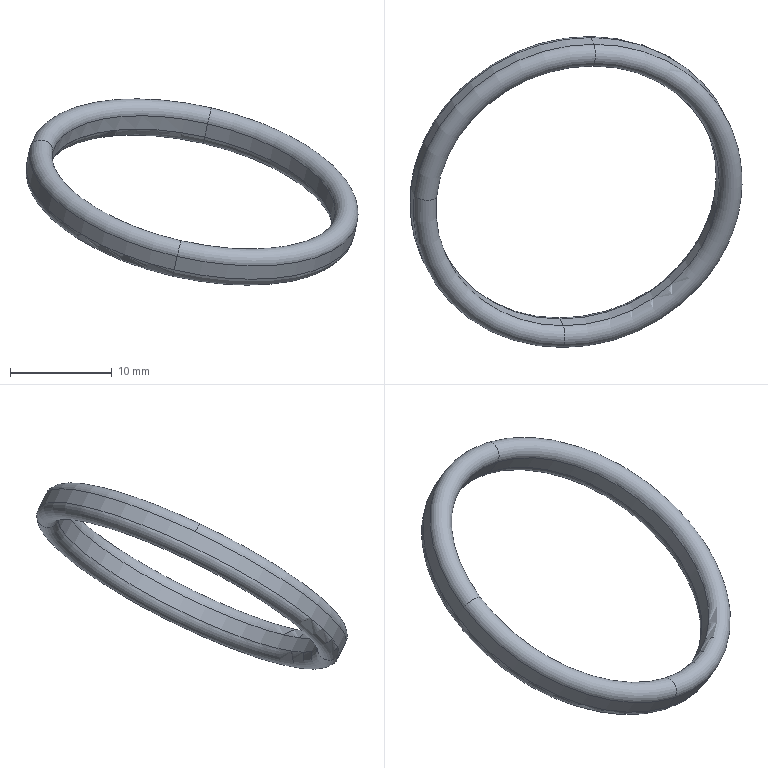Part | SolidWorks | features BaseBody 1 | 1 solid | 9 faces | box 32.672 x 30.577 x 18.335 mm | volume 710.143 mm3 | torus 5 | cylinder 4 | commonest cylinder face diameters 28.5 x2 33 x2
STEP:
#1=CARTESIAN_POINT('',(1913.766,-164.282,837.196));
#2=VERTEX_POINT('',#1);
#3=CARTESIAN_POINT('',(1931.458,-149.433,840.514));
#4=VERTEX_POINT('',#3);
#5=CARTESIAN_POINT('',(1929.847,-164.282,833.502));
#6=DIRECTION('',(-0.2015,0.436,-0.8771));
#7=DIRECTION('',(-0.09761,-0.8999,-0.425));
#8=AXIS2_PLACEMENT_3D('',#5,#6,#7);
#9=CIRCLE('',#8,16.5);
#10=EDGE_CURVE('',#2,#4,#9,.T.);
#11=ORIENTED_EDGE('',*,*,#10,.F.);
#12=CARTESIAN_POINT('',(1915.959,-164.282,836.693));
#13=VERTEX_POINT('',#12);
#14=CARTESIAN_POINT('',(1914.863,-164.282,836.944));
#15=DIRECTION('',(0.09761,0.8999,0.425));
#16=DIRECTION('',(0.,-0.427,0.9043));
#17=AXIS2_PLACEMENT_3D('',#14,#15,#16);
#18=CIRCLE('',#17,1.125);
#19=EDGE_CURVE('',#2,#13,#18,.T.);
#20=ORIENTED_EDGE('',*,*,#19,.T.);
#21=CARTESIAN_POINT('',(1931.238,-151.458,839.558));
#22=VERTEX_POINT('',#21);
#23=CARTESIAN_POINT('',(1929.847,-164.282,833.502));
#24=DIRECTION('',(-0.2015,0.436,-0.8771));
#25=DIRECTION('',(-0.09761,-0.8999,-0.425));
#26=AXIS2_PLACEMENT_3D('',#23,#24,#25);
#27=CIRCLE('',#26,14.25);
#28=EDGE_CURVE('',#13,#22,#27,.T.);
#29=ORIENTED_EDGE('',*,*,#28,.T.);
#30=CARTESIAN_POINT('',(1931.348,-150.445,840.036));
#31=DIRECTION('',(0.9746,0.,-0.2239));
#32=DIRECTION('',(-0.09761,-0.8999,-0.425));
#33=AXIS2_PLACEMENT_3D('',#30,#31,#32);
#34=CIRCLE('',#33,1.125);
#35=EDGE_CURVE('',#4,#22,#34,.T.);
#36=ORIENTED_EDGE('',*,*,#35,.F.);
#37=EDGE_LOOP('',(#11,#20,#29,#36));
#38=FACE_OUTER_BOUND('',#37,.T.);
#39=CARTESIAN_POINT('',(1929.847,-164.282,833.502));
#40=DIRECTION('',(0.2015,-0.436,0.8771));
#41=DIRECTION('',(-0.9746,0.,0.2239));
#42=AXIS2_PLACEMENT_3D('',#39,#40,#41);
#43=TOROIDAL_SURFACE('',#42,15.375,1.125);
#44=ADVANCED_FACE('',(#38),#43,.T.);
#45=CARTESIAN_POINT('',(1928.237,-179.131,826.491));
#46=VERTEX_POINT('',#45);
#47=CARTESIAN_POINT('',(1929.847,-164.282,833.502));
#48=DIRECTION('',(0.2015,-0.436,0.8771));
#49=DIRECTION('',(-0.09761,-0.8999,-0.425));
#50=AXIS2_PLACEMENT_3D('',#47,#48,#49);
#51=CIRCLE('',#50,16.5);
#52=EDGE_CURVE('',#46,#4,#51,.T.);
#53=ORIENTED_EDGE('',*,*,#52,.T.);
#54=ORIENTED_EDGE('',*,*,#35,.T.);
#55=CARTESIAN_POINT('',(1928.457,-177.106,827.447));
#56=VERTEX_POINT('',#55);
#57=CARTESIAN_POINT('',(1929.847,-164.282,833.502));
#58=DIRECTION('',(0.2015,-0.436,0.8771));
#59=DIRECTION('',(-0.09761,-0.8999,-0.425));
#60=AXIS2_PLACEMENT_3D('',#57,#58,#59);
#61=CIRCLE('',#60,14.25);
#62=EDGE_CURVE('',#56,#22,#61,.T.);
#63=ORIENTED_EDGE('',*,*,#62,.F.);
#64=CARTESIAN_POINT('',(1928.347,-178.119,826.969));
#65=DIRECTION('',(0.9746,0.,-0.2239));
#66=DIRECTION('',(0.09761,0.8999,0.425));
#67=AXIS2_PLACEMENT_3D('',#64,#65,#66);
#68=CIRCLE('',#67,1.125);
#69=EDGE_CURVE('',#56,#46,#68,.T.);
#70=ORIENTED_EDGE('',*,*,#69,.T.);
#71=EDGE_LOOP('',(#53,#54,#63,#70));
#72=FACE_OUTER_BOUND('',#71,.T.);
#73=CARTESIAN_POINT('',(1929.847,-164.282,833.502));
#74=DIRECTION('',(0.2015,-0.436,0.8771));
#75=DIRECTION('',(-0.9746,0.,0.2239));
#76=AXIS2_PLACEMENT_3D('',#73,#74,#75);
#77=TOROIDAL_SURFACE('',#76,15.375,1.125);
#78=ADVANCED_FACE('',(#72),#77,.T.);
#79=ORIENTED_EDGE('',*,*,#19,.F.);
#80=CARTESIAN_POINT('',(1929.847,-164.282,833.502));
#81=DIRECTION('',(-0.2015,0.436,-0.8771));
#82=DIRECTION('',(-0.09761,-0.8999,-0.425));
#83=AXIS2_PLACEMENT_3D('',#80,#81,#82);
#84=CIRCLE('',#83,16.5);
#85=EDGE_CURVE('',#46,#2,#84,.T.);
#86=ORIENTED_EDGE('',*,*,#85,.F.);
#87=ORIENTED_EDGE('',*,*,#69,.F.);
#88=CARTESIAN_POINT('',(1929.847,-164.282,833.502));
#89=DIRECTION('',(-0.2015,0.436,-0.8771));
#90=DIRECTION('',(-0.09761,-0.8999,-0.425));
#91=AXIS2_PLACEMENT_3D('',#88,#89,#90);
#92=CIRCLE('',#91,14.25);
#93=EDGE_CURVE('',#56,#13,#92,.T.);
#94=ORIENTED_EDGE('',*,*,#93,.T.);
#95=EDGE_LOOP('',(#79,#86,#87,#94));
#96=FACE_OUTER_BOUND('',#95,.T.);
#97=CARTESIAN_POINT('',(1929.847,-164.282,833.502));
#98=DIRECTION('',(0.2015,-0.436,0.8771));
#99=DIRECTION('',(-0.9746,0.,0.2239));
#100=AXIS2_PLACEMENT_3D('',#97,#98,#99);
#101=TOROIDAL_SURFACE('',#100,15.375,1.125);
#102=ADVANCED_FACE('',(#96),#101,.T.);
#103=ORIENTED_EDGE('',*,*,#85,.T.);
#104=ORIENTED_EDGE('',*,*,#10,.T.);
#105=CARTESIAN_POINT('',(1931.156,-148.779,839.198));
#106=VERTEX_POINT('',#105);
#107=CARTESIAN_POINT('',(1931.458,-149.433,840.514));
#108=DIRECTION('',(0.2015,-0.436,0.8771));
#109=VECTOR('',#108,1000.);
#110=LINE('',#107,#109);
#111=EDGE_CURVE('',#106,#4,#110,.T.);
#112=ORIENTED_EDGE('',*,*,#111,.F.);
#113=CARTESIAN_POINT('',(1927.935,-178.477,825.175));
#114=VERTEX_POINT('',#113);
#115=CARTESIAN_POINT('',(1929.545,-163.628,832.187));
#116=DIRECTION('',(-0.2015,0.436,-0.8771));
#117=DIRECTION('',(-0.09761,-0.8999,-0.425));
#118=AXIS2_PLACEMENT_3D('',#115,#116,#117);
#119=CIRCLE('',#118,16.5);
#120=EDGE_CURVE('',#114,#106,#119,.T.);
#121=ORIENTED_EDGE('',*,*,#120,.F.);
#122=CARTESIAN_POINT('',(1928.237,-179.131,826.491));
#123=DIRECTION('',(-0.2015,0.436,-0.8771));
#124=VECTOR('',#123,1000.);
#125=LINE('',#122,#124);
#126=EDGE_CURVE('',#46,#114,#125,.T.);
#127=ORIENTED_EDGE('',*,*,#126,.F.);
#128=EDGE_LOOP('',(#103,#104,#112,#121,#127));
#129=FACE_OUTER_BOUND('',#128,.T.);
#130=CARTESIAN_POINT('',(1929.521,-163.576,832.081));
#131=DIRECTION('',(0.2015,-0.436,0.8771));
#132=DIRECTION('',(-0.09761,-0.8999,-0.425));
#133=AXIS2_PLACEMENT_3D('',#130,#131,#132);
#134=CYLINDRICAL_SURFACE('',#133,16.5);
#135=ADVANCED_FACE('',(#129),#134,.T.);
#136=CARTESIAN_POINT('',(1929.545,-163.628,832.187));
#137=DIRECTION('',(0.2015,-0.436,0.8771));
#138=DIRECTION('',(-0.09761,-0.8999,-0.425));
#139=AXIS2_PLACEMENT_3D('',#136,#137,#138);
#140=CIRCLE('',#139,16.5);
#141=EDGE_CURVE('',#114,#106,#140,.T.);
#142=ORIENTED_EDGE('',*,*,#141,.T.);
#143=ORIENTED_EDGE('',*,*,#111,.T.);
#144=ORIENTED_EDGE('',*,*,#52,.F.);
#145=ORIENTED_EDGE('',*,*,#126,.T.);
#146=EDGE_LOOP('',(#142,#143,#144,#145));
#147=FACE_OUTER_BOUND('',#146,.T.);
#148=CARTESIAN_POINT('',(1929.521,-163.576,832.081));
#149=DIRECTION('',(0.2015,-0.436,0.8771));
#150=DIRECTION('',(-0.09761,-0.8999,-0.425));
#151=AXIS2_PLACEMENT_3D('',#148,#149,#150);
#152=CYLINDRICAL_SURFACE('',#151,16.5);
#153=ADVANCED_FACE('',(#147),#152,.T.);
#154=CARTESIAN_POINT('',(1928.154,-176.452,826.131));
#155=VERTEX_POINT('',#154);
#156=CARTESIAN_POINT('',(1930.936,-150.804,838.242));
#157=VERTEX_POINT('',#156);
#158=CARTESIAN_POINT('',(1929.545,-163.628,832.187));
#159=DIRECTION('',(0.2015,-0.436,0.8771));
#160=DIRECTION('',(-0.09761,-0.8999,-0.425));
#161=AXIS2_PLACEMENT_3D('',#158,#159,#160);
#162=CIRCLE('',#161,14.25);
#163=EDGE_CURVE('',#155,#157,#162,.T.);
#164=ORIENTED_EDGE('',*,*,#163,.T.);
#165=CARTESIAN_POINT('',(1931.046,-149.791,838.72));
#166=DIRECTION('',(0.9746,0.,-0.2239));
#167=DIRECTION('',(0.09761,0.8999,0.425));
#168=AXIS2_PLACEMENT_3D('',#165,#166,#167);
#169=CIRCLE('',#168,1.125);
#170=EDGE_CURVE('',#157,#106,#169,.T.);
#171=ORIENTED_EDGE('',*,*,#170,.T.);
#172=ORIENTED_EDGE('',*,*,#141,.F.);
#173=CARTESIAN_POINT('',(1928.045,-177.465,825.653));
#174=DIRECTION('',(0.9746,0.,-0.2239));
#175=DIRECTION('',(-0.09761,-0.8999,-0.425));
#176=AXIS2_PLACEMENT_3D('',#173,#174,#175);
#177=CIRCLE('',#176,1.125);
#178=EDGE_CURVE('',#114,#155,#177,.T.);
#179=ORIENTED_EDGE('',*,*,#178,.T.);
#180=EDGE_LOOP('',(#164,#171,#172,#179));
#181=FACE_OUTER_BOUND('',#180,.T.);
#182=CARTESIAN_POINT('',(1929.545,-163.628,832.187));
#183=DIRECTION('',(0.2015,-0.436,0.8771));
#184=DIRECTION('',(-0.09761,-0.8999,-0.425));
#185=AXIS2_PLACEMENT_3D('',#182,#183,#184);
#186=TOROIDAL_SURFACE('',#185,15.375,1.125);
#187=ADVANCED_FACE('',(#181),#186,.T.);
#188=ORIENTED_EDGE('',*,*,#120,.T.);
#189=ORIENTED_EDGE('',*,*,#170,.F.);
#190=CARTESIAN_POINT('',(1929.545,-163.628,832.187));
#191=DIRECTION('',(-0.2015,0.436,-0.8771));
#192=DIRECTION('',(-0.09761,-0.8999,-0.425));
#193=AXIS2_PLACEMENT_3D('',#190,#191,#192);
#194=CIRCLE('',#193,14.25);
#195=EDGE_CURVE('',#155,#157,#194,.T.);
#196=ORIENTED_EDGE('',*,*,#195,.F.);
#197=ORIENTED_EDGE('',*,*,#178,.F.);
#198=EDGE_LOOP('',(#188,#189,#196,#197));
#199=FACE_OUTER_BOUND('',#198,.T.);
#200=CARTESIAN_POINT('',(1929.545,-163.628,832.187));
#201=DIRECTION('',(0.2015,-0.436,0.8771));
#202=DIRECTION('',(-0.09761,-0.8999,-0.425));
#203=AXIS2_PLACEMENT_3D('',#200,#201,#202);
#204=TOROIDAL_SURFACE('',#203,15.375,1.125);
#205=ADVANCED_FACE('',(#199),#204,.T.);
#206=ORIENTED_EDGE('',*,*,#195,.T.);
#207=CARTESIAN_POINT('',(1930.936,-150.804,838.242));
#208=DIRECTION('',(-0.2015,0.436,-0.8771));
#209=VECTOR('',#208,1000.);
#210=LINE('',#207,#209);
#211=EDGE_CURVE('',#22,#157,#210,.T.);
#212=ORIENTED_EDGE('',*,*,#211,.F.);
#213=ORIENTED_EDGE('',*,*,#28,.F.);
#214=ORIENTED_EDGE('',*,*,#93,.F.);
#215=CARTESIAN_POINT('',(1928.154,-176.452,826.131));
#216=DIRECTION('',(0.2015,-0.436,0.8771));
#217=VECTOR('',#216,1000.);
#218=LINE('',#215,#217);
#219=EDGE_CURVE('',#155,#56,#218,.T.);
#220=ORIENTED_EDGE('',*,*,#219,.F.);
#221=EDGE_LOOP('',(#206,#212,#213,#214,#220));
#222=FACE_OUTER_BOUND('',#221,.T.);
#223=CARTESIAN_POINT('',(1929.521,-163.576,832.081));
#224=DIRECTION('',(0.2015,-0.436,0.8771));
#225=DIRECTION('',(-0.09761,-0.8999,-0.425));
#226=AXIS2_PLACEMENT_3D('',#223,#224,#225);
#227=CYLINDRICAL_SURFACE('',#226,14.25);
#228=ADVANCED_FACE('',(#222),#227,.F.);
#229=ORIENTED_EDGE('',*,*,#62,.T.);
#230=ORIENTED_EDGE('',*,*,#211,.T.);
#231=ORIENTED_EDGE('',*,*,#163,.F.);
#232=ORIENTED_EDGE('',*,*,#219,.T.);
#233=EDGE_LOOP('',(#229,#230,#231,#232));
#234=FACE_OUTER_BOUND('',#233,.T.);
#235=CARTESIAN_POINT('',(1929.521,-163.576,832.081));
#236=DIRECTION('',(0.2015,-0.436,0.8771));
#237=DIRECTION('',(-0.09761,-0.8999,-0.425));
#238=AXIS2_PLACEMENT_3D('',#235,#236,#237);
#239=CYLINDRICAL_SURFACE('',#238,14.25);
#240=ADVANCED_FACE('',(#234),#239,.F.);
#241=CLOSED_SHELL('',(#44,#78,#102,#135,#153,#187,#205,#228,#240));
#242=MANIFOLD_SOLID_BREP('',#241);
#243=CARTESIAN_POINT('',(0.,0.,0.));
#244=DIRECTION('',(0.,0.,1.));
#245=DIRECTION('',(1.,0.,0.));
#246=AXIS2_PLACEMENT_3D('',#243,#244,#245);
#247=(LENGTH_UNIT()NAMED_UNIT(*)SI_UNIT(.MILLI.,.METRE.));
#248=UNCERTAINTY_MEASURE_WITH_UNIT(LENGTH_MEASURE(0.00001),#247,'','');
#249=(NAMED_UNIT(*)PLANE_ANGLE_UNIT()SI_UNIT($,.RADIAN.));
#250=(NAMED_UNIT(*)SI_UNIT($,.STERADIAN.)SOLID_ANGLE_UNIT());
#251=(GEOMETRIC_REPRESENTATION_CONTEXT(3)GLOBAL_UNCERTAINTY_ASSIGNED_CONTEXT((#248))GLOBAL_UNIT_ASSIGNED_CONTEXT((#247,#249,#250))REPRESENTATION_CONTEXT('',''));
#252=ADVANCED_BREP_SHAPE_REPRESENTATION('',(#242,#246),#251);